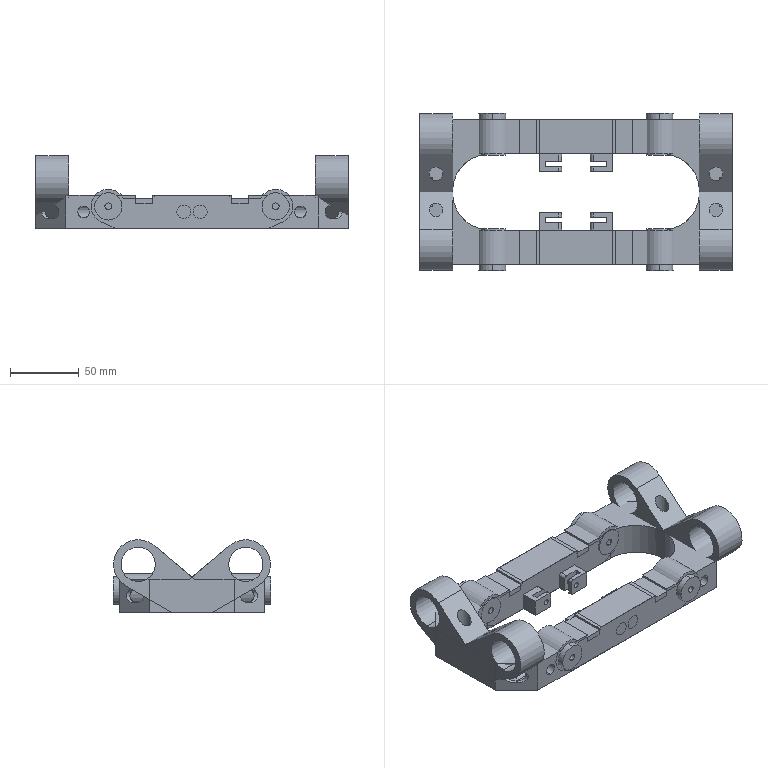NC program | Mastercam | posted with a generic post | part box 228 x 114.503 x 53 mm
Lines 1813 to 2707 of 27132:
(50 FEM |TOOL - 23|DIA. OFF. - 23|LEN. - 23|TOOL DIA. - 50.)
N3680 T23 M6
N3682 G0 G54 G90 X92.548 Y31.5 C0. B0. S5000 M3
N3684 G43 H23 Z50.
N3686 Z5.
N3688 G1 Z-.5 F600.
N3690 X87.548 F4000.
N3692 G3 X82.548 Y26.5 J-5.
N3694 G1 Y2.5
N3696 G2 X57.248 Y-22.8 I-25.3
N3698 G1 X11.069
N3700 X-11.419 Y-41.67
N3702 G2 X-39.252 Y-51.8 I-27.833 J33.17
N3704 X-82.552 Y-8.5 J43.3
N3706 X-60.902 Y28.999 I43.3
N3708 G1 X-21.409 Y51.8
N3710 X57.248
N3712 G2 X82.548 Y26.5 J-25.3
N3714 G1 Y21.5
N3716 G3 X87.548 Y16.5 I5.
N3718 G1 X92.548
N3720 Y31.5
N3722 Z-1. F600.
N3724 X87.548 F4000.
N3726 G3 X82.548 Y26.5 J-5.
N3728 G1 Y2.5
N3730 G2 X57.248 Y-22.8 I-25.3
N3732 G1 X11.069
N3734 X-11.419 Y-41.67
N3736 G2 X-39.252 Y-51.8 I-27.833 J33.17
N3738 X-82.552 Y-8.5 J43.3
N3740 X-60.902 Y28.999 I43.3
N3742 G1 X-21.409 Y51.8
N3744 X57.248
N3746 G2 X82.548 Y26.5 J-25.3
N3748 G1 Y21.5
N3750 G3 X87.548 Y16.5 I5.
N3752 G1 X92.548
N3754 Y31.5
N3756 Z-1.5 F600.
N3758 X87.548 F4000.
N3760 G3 X82.548 Y26.5 J-5.
N3762 G1 Y2.5
N3764 G2 X57.248 Y-22.8 I-25.3
N3766 G1 X11.069
N3768 X-11.419 Y-41.67
N3770 G2 X-39.252 Y-51.8 I-27.833 J33.17
N3772 X-82.552 Y-8.5 J43.3
N3774 X-60.902 Y28.999 I43.3
N3776 G1 X-21.409 Y51.8
N3778 X57.248
N3780 G2 X82.548 Y26.5 J-25.3
N3782 G1 Y21.5
N3784 G3 X87.548 Y16.5 I5.
N3786 G1 X92.548
N3788 Y31.5
N3790 Z-2. F600.
N3792 X87.548 F4000.
N3794 G3 X82.548 Y26.5 J-5.
N3796 G1 Y2.5
N3798 G2 X57.248 Y-22.8 I-25.3
N3800 G1 X11.069
N3802 X-11.419 Y-41.67
N3804 G2 X-39.252 Y-51.8 I-27.833 J33.17
N3806 X-82.552 Y-8.5 J43.3
N3808 X-60.902 Y28.999 I43.3
N3810 G1 X-21.409 Y51.8
N3812 X57.248
N3814 G2 X82.548 Y26.5 J-25.3
N3816 G1 Y21.5
N3818 G3 X87.548 Y16.5 I5.
N3820 G1 X92.548
N3822 Y31.5
N3824 Z-2.5 F600.
N3826 X87.548 F4000.
N3828 G3 X82.548 Y26.5 J-5.
N3830 G1 Y2.5
N3832 G2 X57.248 Y-22.8 I-25.3
N3834 G1 X11.069
N3836 X-11.419 Y-41.67
N3838 G2 X-39.252 Y-51.8 I-27.833 J33.17
N3840 X-82.552 Y-8.5 J43.3
N3842 X-60.902 Y28.999 I43.3
N3844 G1 X-21.409 Y51.8
N3846 X57.248
N3848 G2 X82.548 Y26.5 J-25.3
N3850 G1 Y21.5
N3852 G3 X87.548 Y16.5 I5.
N3854 G1 X92.548
N3856 Y31.5
N3858 Z-3. F600.
N3860 X87.548 F4000.
N3862 G3 X82.548 Y26.5 J-5.
N3864 G1 Y2.5
N3866 G2 X57.248 Y-22.8 I-25.3
N3868 G1 X11.069
N3870 X-11.419 Y-41.67
N3872 G2 X-39.252 Y-51.8 I-27.833 J33.17
N3874 X-82.552 Y-8.5 J43.3
N3876 X-60.902 Y28.999 I43.3
N3878 G1 X-21.409 Y51.8
N3880 X57.248
N3882 G2 X82.548 Y26.5 J-25.3
N3884 G1 Y21.5
N3886 G3 X87.548 Y16.5 I5.
N3888 G1 X92.548
N3890 Y31.5
N3892 Z-3.5 F600.
N3894 X87.548 F4000.
N3896 G3 X82.548 Y26.5 J-5.
N3898 G1 Y2.5
N3900 G2 X57.248 Y-22.8 I-25.3
N3902 G1 X11.069
N3904 X-11.419 Y-41.67
N3906 G2 X-39.252 Y-51.8 I-27.833 J33.17
N3908 X-82.552 Y-8.5 J43.3
N3910 X-60.902 Y28.999 I43.3
N3912 G1 X-21.409 Y51.8
N3914 X57.248
N3916 G2 X82.548 Y26.5 J-25.3
N3918 G1 Y21.5
N3920 G3 X87.548 Y16.5 I5.
N3922 G1 X92.548
N3924 Y31.5
N3926 Z-4. F600.
N3928 X87.548 F4000.
N3930 G3 X82.548 Y26.5 J-5.
N3932 G1 Y2.5
N3934 G2 X57.248 Y-22.8 I-25.3
N3936 G1 X11.069
N3938 X-11.419 Y-41.67
N3940 G2 X-39.252 Y-51.8 I-27.833 J33.17
N3942 X-82.552 Y-8.5 J43.3
N3944 X-60.902 Y28.999 I43.3
N3946 G1 X-21.409 Y51.8
N3948 X57.248
N3950 G2 X82.548 Y26.5 J-25.3
N3952 G1 Y21.5
N3954 G3 X87.548 Y16.5 I5.
N3956 G1 X92.548
N3958 Y31.5
N3960 Z-4.5 F600.
N3962 X87.548 F4000.
N3964 G3 X82.548 Y26.5 J-5.
N3966 G1 Y2.5
N3968 G2 X57.248 Y-22.8 I-25.3
N3970 G1 X11.069
N3972 X-11.419 Y-41.67
N3974 G2 X-39.252 Y-51.8 I-27.833 J33.17
N3976 X-82.552 Y-8.5 J43.3
N3978 X-60.902 Y28.999 I43.3
N3980 G1 X-21.409 Y51.8
N3982 X57.248
N3984 G2 X82.548 Y26.5 J-25.3
N3986 G1 Y21.5
N3988 G3 X87.548 Y16.5 I5.
N3990 G1 X92.548
N3992 Y31.5
N3994 Z-5. F600.
N3996 X87.548 F4000.
N3998 G3 X82.548 Y26.5 J-5.
N4000 G1 Y2.5
N4002 G2 X57.248 Y-22.8 I-25.3
N4004 G1 X11.069
N4006 X-11.419 Y-41.67
N4008 G2 X-39.252 Y-51.8 I-27.833 J33.17
N4010 X-82.552 Y-8.5 J43.3
N4012 X-60.902 Y28.999 I43.3
N4014 G1 X-21.409 Y51.8
N4016 X57.248
N4018 G2 X82.548 Y26.5 J-25.3
N4020 G1 Y21.5
N4022 G3 X87.548 Y16.5 I5.
N4024 G1 X92.548
N4026 Y31.5
N4028 Z-5.5 F600.
N4030 X87.548 F4000.
N4032 G3 X82.548 Y26.5 J-5.
N4034 G1 Y2.5
N4036 G2 X57.248 Y-22.8 I-25.3
N4038 G1 X11.069
N4040 X-11.419 Y-41.67
N4042 G2 X-39.252 Y-51.8 I-27.833 J33.17
N4044 X-82.552 Y-8.5 J43.3
N4046 X-60.902 Y28.999 I43.3
N4048 G1 X-21.409 Y51.8
N4050 X57.248
N4052 G2 X82.548 Y26.5 J-25.3
N4054 G1 Y21.5
N4056 G3 X87.548 Y16.5 I5.
N4058 G1 X92.548
N4060 Y31.5
N4062 Z-6. F600.
N4064 X87.548 F4000.
N4066 G3 X82.548 Y26.5 J-5.
N4068 G1 Y2.5
N4070 G2 X57.248 Y-22.8 I-25.3
N4072 G1 X11.069
N4074 X-11.419 Y-41.67
N4076 G2 X-39.252 Y-51.8 I-27.833 J33.17
N4078 X-82.552 Y-8.5 J43.3
N4080 X-60.902 Y28.999 I43.3
N4082 G1 X-21.409 Y51.8
N4084 X57.248
N4086 G2 X82.548 Y26.5 J-25.3
N4088 G1 Y21.5
N4090 G3 X87.548 Y16.5 I5.
N4092 G1 X92.548
N4094 Y31.5
N4096 Z-6.5 F600.
N4098 X87.548 F4000.
N4100 G3 X82.548 Y26.5 J-5.
N4102 G1 Y2.5
N4104 G2 X57.248 Y-22.8 I-25.3
N4106 G1 X11.069
N4108 X-11.419 Y-41.67
N4110 G2 X-39.252 Y-51.8 I-27.833 J33.17
N4112 X-82.552 Y-8.5 J43.3
N4114 X-60.902 Y28.999 I43.3
N4116 G1 X-21.409 Y51.8
N4118 X57.248
N4120 G2 X82.548 Y26.5 J-25.3
N4122 G1 Y21.5
N4124 G3 X87.548 Y16.5 I5.
N4126 G1 X92.548
N4128 Y31.5
N4130 Z-7. F600.
N4132 X87.548 F4000.
N4134 G3 X82.548 Y26.5 J-5.
N4136 G1 Y2.5
N4138 G2 X57.248 Y-22.8 I-25.3
N4140 G1 X11.069
N4142 X-11.419 Y-41.67
N4144 G2 X-39.252 Y-51.8 I-27.833 J33.17
N4146 X-82.552 Y-8.5 J43.3
N4148 X-60.902 Y28.999 I43.3
N4150 G1 X-21.409 Y51.8
N4152 X57.248
N4154 G2 X82.548 Y26.5 J-25.3
N4156 G1 Y21.5
N4158 G3 X87.548 Y16.5 I5.
N4160 G1 X92.548
N4162 Y31.5
N4164 Z-7.5 F600.
N4166 X87.548 F4000.
N4168 G3 X82.548 Y26.5 J-5.
N4170 G1 Y2.5
N4172 G2 X57.248 Y-22.8 I-25.3
N4174 G1 X11.069
N4176 X-11.419 Y-41.67
N4178 G2 X-39.252 Y-51.8 I-27.833 J33.17
N4180 X-82.552 Y-8.5 J43.3
N4182 X-60.902 Y28.999 I43.3
N4184 G1 X-21.409 Y51.8
N4186 X57.248
N4188 G2 X82.548 Y26.5 J-25.3
N4190 G1 Y21.5
N4192 G3 X87.548 Y16.5 I5.
N4194 G1 X92.548
N4196 Y31.5
N4198 Z-8. F600.
N4200 X87.548 F4000.
N4202 G3 X82.548 Y26.5 J-5.
N4204 G1 Y2.5
N4206 G2 X57.248 Y-22.8 I-25.3
N4208 G1 X11.069
N4210 X-11.419 Y-41.67
N4212 G2 X-39.252 Y-51.8 I-27.833 J33.17
N4214 X-82.552 Y-8.5 J43.3
N4216 X-60.902 Y28.999 I43.3
N4218 G1 X-21.409 Y51.8
N4220 X57.248
N4222 G2 X82.548 Y26.5 J-25.3
N4224 G1 Y21.5
N4226 G3 X87.548 Y16.5 I5.
N4228 G1 X92.548
N4230 Y31.5
N4232 Z-8.5 F600.
N4234 X87.548 F4000.
N4236 G3 X82.548 Y26.5 J-5.
N4238 G1 Y2.5
N4240 G2 X57.248 Y-22.8 I-25.3
N4242 G1 X11.069
N4244 X-11.419 Y-41.67
N4246 G2 X-39.252 Y-51.8 I-27.833 J33.17
N4248 X-82.552 Y-8.5 J43.3
N4250 X-60.902 Y28.999 I43.3
N4252 G1 X-21.409 Y51.8
N4254 X57.248
N4256 G2 X82.548 Y26.5 J-25.3
N4258 G1 Y21.5
N4260 G3 X87.548 Y16.5 I5.
N4262 G1 X92.548
N4264 Y31.5
N4266 Z-9. F600.
N4268 X87.548 F4000.
N4270 G3 X82.548 Y26.5 J-5.
N4272 G1 Y2.5
N4274 G2 X57.248 Y-22.8 I-25.3
N4276 G1 X11.069
N4278 X-11.419 Y-41.67
N4280 G2 X-39.252 Y-51.8 I-27.833 J33.17
N4282 X-82.552 Y-8.5 J43.3
N4284 X-60.902 Y28.999 I43.3
N4286 G1 X-21.409 Y51.8
N4288 X57.248
N4290 G2 X82.548 Y26.5 J-25.3
N4292 G1 Y21.5
N4294 G3 X87.548 Y16.5 I5.
N4296 G1 X92.548
N4298 Y31.5
N4300 Z-9.5 F600.
N4302 X87.548 F4000.
N4304 G3 X82.548 Y26.5 J-5.
N4306 G1 Y2.5
N4308 G2 X57.248 Y-22.8 I-25.3
N4310 G1 X11.069
N4312 X-11.419 Y-41.67
N4314 G2 X-39.252 Y-51.8 I-27.833 J33.17
N4316 X-82.552 Y-8.5 J43.3
N4318 X-60.902 Y28.999 I43.3
N4320 G1 X-21.409 Y51.8
N4322 X57.248
N4324 G2 X82.548 Y26.5 J-25.3
N4326 G1 Y21.5
N4328 G3 X87.548 Y16.5 I5.
N4330 G1 X92.548
N4332 Y31.5
N4334 Z-10. F600.
N4336 X87.548 F4000.
N4338 G3 X82.548 Y26.5 J-5.
N4340 G1 Y2.5
N4342 G2 X57.248 Y-22.8 I-25.3
N4344 G1 X11.069
N4346 X-11.419 Y-41.67
N4348 G2 X-39.252 Y-51.8 I-27.833 J33.17
N4350 X-82.552 Y-8.5 J43.3
N4352 X-60.902 Y28.999 I43.3
N4354 G1 X-21.409 Y51.8
N4356 X57.248
N4358 G2 X82.548 Y26.5 J-25.3
N4360 G1 Y21.5
N4362 G3 X87.548 Y16.5 I5.
N4364 G1 X92.548
N4366 Y31.5
N4368 Z-10.5 F600.
N4370 X87.548 F4000.
N4372 G3 X82.548 Y26.5 J-5.
N4374 G1 Y2.5
N4376 G2 X57.248 Y-22.8 I-25.3
N4378 G1 X11.069
N4380 X-11.419 Y-41.67
N4382 G2 X-39.252 Y-51.8 I-27.833 J33.17
N4384 X-82.552 Y-8.5 J43.3
N4386 X-60.902 Y28.999 I43.3
N4388 G1 X-21.409 Y51.8
N4390 X57.248
N4392 G2 X82.548 Y26.5 J-25.3
N4394 G1 Y21.5
N4396 G3 X87.548 Y16.5 I5.
N4398 G1 X92.548
N4400 Y31.5
N4402 Z-11. F600.
N4404 X87.548 F4000.
N4406 G3 X82.548 Y26.5 J-5.
N4408 G1 Y2.5
N4410 G2 X57.248 Y-22.8 I-25.3
N4412 G1 X11.069
N4414 X-11.419 Y-41.67
N4416 G2 X-39.252 Y-51.8 I-27.833 J33.17
N4418 X-82.552 Y-8.5 J43.3
N4420 X-60.902 Y28.999 I43.3
N4422 G1 X-21.409 Y51.8
N4424 X57.248
N4426 G2 X82.548 Y26.5 J-25.3
N4428 G1 Y21.5
N4430 G3 X87.548 Y16.5 I5.
N4432 G1 X92.548
N4434 Y31.5
N4436 Z-11.5 F600.
N4438 X87.548 F4000.
N4440 G3 X82.548 Y26.5 J-5.
N4442 G1 Y2.5
N4444 G2 X57.248 Y-22.8 I-25.3
N4446 G1 X11.069
N4448 X-11.419 Y-41.67
N4450 G2 X-39.252 Y-51.8 I-27.833 J33.17
N4452 X-82.552 Y-8.5 J43.3
N4454 X-60.902 Y28.999 I43.3
N4456 G1 X-21.409 Y51.8
N4458 X57.248
N4460 G2 X82.548 Y26.5 J-25.3
N4462 G1 Y21.5
N4464 G3 X87.548 Y16.5 I5.
N4466 G1 X92.548
N4468 Y31.5
N4470 Z-12. F600.
N4472 X87.548 F4000.
N4474 G3 X82.548 Y26.5 J-5.
N4476 G1 Y2.5
N4478 G2 X57.248 Y-22.8 I-25.3
N4480 G1 X11.069
N4482 X-11.419 Y-41.67
N4484 G2 X-39.252 Y-51.8 I-27.833 J33.17
N4486 X-82.552 Y-8.5 J43.3
N4488 X-60.902 Y28.999 I43.3
N4490 G1 X-21.409 Y51.8
N4492 X57.248
N4494 G2 X82.548 Y26.5 J-25.3
N4496 G1 Y21.5
N4498 G3 X87.548 Y16.5 I5.
N4500 G1 X92.548
N4502 Y31.5
N4504 Z-12.5 F600.
N4506 X87.548 F4000.
N4508 G3 X82.548 Y26.5 J-5.
N4510 G1 Y2.5
N4512 G2 X57.248 Y-22.8 I-25.3
N4514 G1 X11.069
N4516 X-11.419 Y-41.67
N4518 G2 X-39.252 Y-51.8 I-27.833 J33.17
N4520 X-82.552 Y-8.5 J43.3
N4522 X-60.902 Y28.999 I43.3
N4524 G1 X-21.409 Y51.8
N4526 X57.248
N4528 G2 X82.548 Y26.5 J-25.3
N4530 G1 Y21.5
N4532 G3 X87.548 Y16.5 I5.
N4534 G1 X92.548
N4536 Y31.5
N4538 Z-13. F600.
N4540 X87.548 F4000.
N4542 G3 X82.548 Y26.5 J-5.
N4544 G1 Y2.5
N4546 G2 X57.248 Y-22.8 I-25.3
N4548 G1 X11.069
N4550 X-11.419 Y-41.67
N4552 G2 X-39.252 Y-51.8 I-27.833 J33.17
N4554 X-82.552 Y-8.5 J43.3
N4556 X-60.902 Y28.999 I43.3
N4558 G1 X-21.409 Y51.8
N4560 X57.248
N4562 G2 X82.548 Y26.5 J-25.3
N4564 G1 Y21.5
N4566 G3 X87.548 Y16.5 I5.
N4568 G1 X92.548
N4570 Y31.5
N4572 Z-13.5 F600.
N4574 X87.548 F4000.
N4576 G3 X82.548 Y26.5 J-5.
N4578 G1 Y2.5
N4580 G2 X57.248 Y-22.8 I-25.3
N4582 G1 X11.069
N4584 X-11.419 Y-41.67
N4586 G2 X-39.252 Y-51.8 I-27.833 J33.17
N4588 X-82.552 Y-8.5 J43.3
N4590 X-60.902 Y28.999 I43.3
N4592 G1 X-21.409 Y51.8
N4594 X57.248
N4596 G2 X82.548 Y26.5 J-25.3
N4598 G1 Y21.5
N4600 G3 X87.548 Y16.5 I5.
N4602 G1 X92.548
N4604 Y31.5
N4606 Z-14. F600.
N4608 X87.548 F4000.
N4610 G3 X82.548 Y26.5 J-5.
N4612 G1 Y2.5
N4614 G2 X57.248 Y-22.8 I-25.3
N4616 G1 X11.069
N4618 X-11.419 Y-41.67
N4620 G2 X-39.252 Y-51.8 I-27.833 J33.17
N4622 X-82.552 Y-8.5 J43.3
N4624 X-60.902 Y28.999 I43.3
N4626 G1 X-21.409 Y51.8
N4628 X57.248
N4630 G2 X82.548 Y26.5 J-25.3
N4632 G1 Y21.5
N4634 G3 X87.548 Y16.5 I5.
N4636 G1 X92.548
N4638 Y31.5
N4640 Z-14.5 F600.
N4642 X87.548 F4000.
N4644 G3 X82.548 Y26.5 J-5.
N4646 G1 Y2.5
N4648 G2 X57.248 Y-22.8 I-25.3
N4650 G1 X11.069
N4652 X-11.419 Y-41.67
N4654 G2 X-39.252 Y-51.8 I-27.833 J33.17
N4656 X-82.552 Y-8.5 J43.3
N4658 X-60.902 Y28.999 I43.3
N4660 G1 X-21.409 Y51.8
N4662 X57.248
N4664 G2 X82.548 Y26.5 J-25.3
N4666 G1 Y21.5
N4668 G3 X87.548 Y16.5 I5.
N4670 G1 X92.548
N4672 Y31.5
N4674 Z-15. F600.
N4676 X87.548 F4000.
N4678 G3 X82.548 Y26.5 J-5.
N4680 G1 Y2.5
N4682 G2 X57.248 Y-22.8 I-25.3
N4684 G1 X11.069
N4686 X-11.419 Y-41.67
N4688 G2 X-39.252 Y-51.8 I-27.833 J33.17
N4690 X-82.552 Y-8.5 J43.3
N4692 X-60.902 Y28.999 I43.3
N4694 G1 X-21.409 Y51.8
N4696 X57.248
N4698 G2 X82.548 Y26.5 J-25.3
N4700 G1 Y21.5
N4702 G3 X87.548 Y16.5 I5.
N4704 G1 X92.548
N4706 Y31.5
N4708 Z-15.5 F600.
N4710 X87.548 F4000.
N4712 G3 X82.548 Y26.5 J-5.
N4714 G1 Y2.5
N4716 G2 X57.248 Y-22.8 I-25.3
N4718 G1 X11.069
N4720 X-11.419 Y-41.67
N4722 G2 X-39.252 Y-51.8 I-27.833 J33.17
N4724 X-82.552 Y-8.5 J43.3
N4726 X-60.902 Y28.999 I43.3
N4728 G1 X-21.409 Y51.8
N4730 X57.248
N4732 G2 X82.548 Y26.5 J-25.3
N4734 G1 Y21.5
N4736 G3 X87.548 Y16.5 I5.
N4738 G1 X92.548
N4740 Y31.5
N4742 Z-16. F600.
N4744 X87.548 F4000.
N4746 G3 X82.548 Y26.5 J-5.
N4748 G1 Y2.5
N4750 G2 X57.248 Y-22.8 I-25.3
N4752 G1 X11.069
N4754 X-11.419 Y-41.67
N4756 G2 X-39.252 Y-51.8 I-27.833 J33.17
N4758 X-82.552 Y-8.5 J43.3
N4760 X-60.902 Y28.999 I43.3
N4762 G1 X-21.409 Y51.8
N4764 X57.248
N4766 G2 X82.548 Y26.5 J-25.3
N4768 G1 Y21.5
N4770 G3 X87.548 Y16.5 I5.
N4772 G1 X92.548
N4774 Y31.5
N4776 Z-16.5 F600.
N4778 X87.548 F4000.
N4780 G3 X82.548 Y26.5 J-5.
N4782 G1 Y2.5
N4784 G2 X57.248 Y-22.8 I-25.3
N4786 G1 X11.069
N4788 X-11.419 Y-41.67
N4790 G2 X-39.252 Y-51.8 I-27.833 J33.17
N4792 X-82.552 Y-8.5 J43.3
N4794 X-60.902 Y28.999 I43.3
N4796 G1 X-21.409 Y51.8
N4798 X57.248
N4800 G2 X82.548 Y26.5 J-25.3
N4802 G1 Y21.5
N4804 G3 X87.548 Y16.5 I5.
N4806 G1 X92.548
N4808 Y31.5
N4810 Z-17. F600.
N4812 X87.548 F4000.
N4814 G3 X82.548 Y26.5 J-5.
N4816 G1 Y2.5
N4818 G2 X57.248 Y-22.8 I-25.3
N4820 G1 X11.069
N4822 X-11.419 Y-41.67
N4824 G2 X-39.252 Y-51.8 I-27.833 J33.17
N4826 X-82.552 Y-8.5 J43.3
N4828 X-60.902 Y28.999 I43.3
N4830 G1 X-21.409 Y51.8
N4832 X57.248
N4834 G2 X82.548 Y26.5 J-25.3
N4836 G1 Y21.5
N4838 G3 X87.548 Y16.5 I5.
N4840 G1 X92.548
N4842 Y31.5
N4844 Z-17.5 F600.
N4846 X87.548 F4000.
N4848 G3 X82.548 Y26.5 J-5.
N4850 G1 Y2.5
N4852 G2 X57.248 Y-22.8 I-25.3
N4854 G1 X11.069
N4856 X-11.419 Y-41.67
N4858 G2 X-39.252 Y-51.8 I-27.833 J33.17
N4860 X-82.552 Y-8.5 J43.3
N4862 X-60.902 Y28.999 I43.3
N4864 G1 X-21.409 Y51.8
N4866 X57.248
N4868 G2 X82.548 Y26.5 J-25.3
N4870 G1 Y21.5
N4872 G3 X87.548 Y16.5 I5.
N4874 G1 X92.548
N4876 Y31.5
N4878 Z-18. F600.
N4880 X87.548 F4000.
N4882 G3 X82.548 Y26.5 J-5.
N4884 G1 Y2.5
N4886 G2 X57.248 Y-22.8 I-25.3
N4888 G1 X11.069
N4890 X-11.419 Y-41.67
N4892 G2 X-39.252 Y-51.8 I-27.833 J33.17
N4894 X-82.552 Y-8.5 J43.3
N4896 X-60.902 Y28.999 I43.3
N4898 G1 X-21.409 Y51.8
N4900 X57.248
N4902 G2 X82.548 Y26.5 J-25.3
N4904 G1 Y21.5
N4906 G3 X87.548 Y16.5 I5.
N4908 G1 X92.548
N4910 Y31.5
N4912 Z-18.5 F600.
N4914 X87.548 F4000.
N4916 G3 X82.548 Y26.5 J-5.
N4918 G1 Y2.5
N4920 G2 X57.248 Y-22.8 I-25.3
N4922 G1 X11.069
N4924 X-11.419 Y-41.67
N4926 G2 X-39.252 Y-51.8 I-27.833 J33.17
N4928 X-82.552 Y-8.5 J43.3
N4930 X-60.902 Y28.999 I43.3
N4932 G1 X-21.409 Y51.8
N4934 X57.248
N4936 G2 X82.548 Y26.5 J-25.3
N4938 G1 Y21.5
N4940 G3 X87.548 Y16.5 I5.
N4942 G1 X92.548
N4944 Y31.5
N4946 Z-19. F600.
N4948 X87.548 F4000.
N4950 G3 X82.548 Y26.5 J-5.
N4952 G1 Y2.5
N4954 G2 X57.248 Y-22.8 I-25.3
N4956 G1 X11.069
N4958 X-11.419 Y-41.67
N4960 G2 X-39.252 Y-51.8 I-27.833 J33.17
N4962 X-82.552 Y-8.5 J43.3
N4964 X-60.902 Y28.999 I43.3
N4966 G1 X-21.409 Y51.8
N4968 X57.248
N4970 G2 X82.548 Y26.5 J-25.3
N4972 G1 Y21.5
N4974 G3 X87.548 Y16.5 I5.
N4976 G1 X92.548
N4978 Y31.5
N4980 Z-19.5 F600.
N4982 X87.548 F4000.
N4984 G3 X82.548 Y26.5 J-5.
N4986 G1 Y2.5
N4988 G2 X57.248 Y-22.8 I-25.3
N4990 G1 X11.069
N4992 X-11.419 Y-41.67
N4994 G2 X-39.252 Y-51.8 I-27.833 J33.17
N4996 X-82.552 Y-8.5 J43.3
N4998 X-60.902 Y28.999 I43.3
N5000 G1 X-21.409 Y51.8
N5002 X57.248
N5004 G2 X82.548 Y26.5 J-25.3
N5006 G1 Y21.5
N5008 G3 X87.548 Y16.5 I5.
N5010 G1 X92.548
N5012 Y31.5
N5014 Z-20. F600.
N5016 X87.548 F4000.
N5018 G3 X82.548 Y26.5 J-5.
N5020 G1 Y2.5
N5022 G2 X57.248 Y-22.8 I-25.3
N5024 G1 X11.069
N5026 X-11.419 Y-41.67
N5028 G2 X-39.252 Y-51.8 I-27.833 J33.17
N5030 X-82.552 Y-8.5 J43.3
N5032 X-60.902 Y28.999 I43.3
N5034 G1 X-21.409 Y51.8
N5036 X57.248
N5038 G2 X82.548 Y26.5 J-25.3
N5040 G1 Y21.5
N5042 G3 X87.548 Y16.5 I5.
N5044 G1 X92.548
N5046 Y31.5
N5048 Z-20.5 F600.
N5050 X87.548 F4000.
N5052 G3 X82.548 Y26.5 J-5.
N5054 G1 Y2.5
N5056 G2 X57.248 Y-22.8 I-25.3
N5058 G1 X11.069
N5060 X-11.419 Y-41.67
N5062 G2 X-39.252 Y-51.8 I-27.833 J33.17
N5064 X-82.552 Y-8.5 J43.3
N5066 X-60.902 Y28.999 I43.3
N5068 G1 X-21.409 Y51.8
N5070 X57.248
N5072 G2 X82.548 Y26.5 J-25.3
N5074 G1 Y21.5
N5076 G3 X87.548 Y16.5 I5.
N5078 G1 X92.548
N5080 Y31.5
N5082 Z-21. F600.
N5084 X87.548 F4000.
N5086 G3 X82.548 Y26.5 J-5.
N5088 G1 Y2.5
N5090 G2 X57.248 Y-22.8 I-25.3
N5092 G1 X11.069
N5094 X-11.419 Y-41.67
N5096 G2 X-39.252 Y-51.8 I-27.833 J33.17
N5098 X-82.552 Y-8.5 J43.3
N5100 X-60.902 Y28.999 I43.3
N5102 G1 X-21.409 Y51.8
N5104 X57.248
N5106 G2 X82.548 Y26.5 J-25.3
N5108 G1 Y21.5
N5110 G3 X87.548 Y16.5 I5.
N5112 G1 X92.548
N5114 Y31.5
N5116 Z-21.5 F600.
N5118 X87.548 F4000.
N5120 G3 X82.548 Y26.5 J-5.
N5122 G1 Y2.5
N5124 G2 X57.248 Y-22.8 I-25.3
N5126 G1 X11.069
N5128 X-11.419 Y-41.67
N5130 G2 X-39.252 Y-51.8 I-27.833 J33.17
N5132 X-82.552 Y-8.5 J43.3
N5134 X-60.902 Y28.999 I43.3
N5136 G1 X-21.409 Y51.8
N5138 X57.248
N5140 G2 X82.548 Y26.5 J-25.3
N5142 G1 Y21.5
N5144 G3 X87.548 Y16.5 I5.
N5146 G1 X92.548
N5148 Y31.5
N5150 Z-22. F600.
N5152 X87.548 F4000.
N5154 G3 X82.548 Y26.5 J-5.
N5156 G1 Y2.5
N5158 G2 X57.248 Y-22.8 I-25.3
N5160 G1 X11.069
N5162 X-11.419 Y-41.67
N5164 G2 X-39.252 Y-51.8 I-27.833 J33.17
N5166 X-82.552 Y-8.5 J43.3
N5168 X-60.902 Y28.999 I43.3
N5170 G1 X-21.409 Y51.8
N5172 X57.248
N5174 G2 X82.548 Y26.5 J-25.3
N5176 G1 Y21.5
N5178 G3 X87.548 Y16.5 I5.
N5180 G1 X92.548
N5182 Y31.5
N5184 Z-22.5 F600.
N5186 X87.548 F4000.
N5188 G3 X82.548 Y26.5 J-5.
N5190 G1 Y2.5
N5192 G2 X57.248 Y-22.8 I-25.3
N5194 G1 X11.069
N5196 X-11.419 Y-41.67
N5198 G2 X-39.252 Y-51.8 I-27.833 J33.17
N5200 X-82.552 Y-8.5 J43.3
N5202 X-60.902 Y28.999 I43.3
N5204 G1 X-21.409 Y51.8
N5206 X57.248
N5208 G2 X82.548 Y26.5 J-25.3
N5210 G1 Y21.5
N5212 G3 X87.548 Y16.5 I5.
N5214 G1 X92.548
N5216 Y31.5
N5218 Z-23. F600.
N5220 X87.548 F4000.
N5222 G3 X82.548 Y26.5 J-5.
N5224 G1 Y2.5
N5226 G2 X57.248 Y-22.8 I-25.3
N5228 G1 X11.069
N5230 X-11.419 Y-41.67
N5232 G2 X-39.252 Y-51.8 I-27.833 J33.17
N5234 X-82.552 Y-8.5 J43.3
N5236 X-60.902 Y28.999 I43.3
N5238 G1 X-21.409 Y51.8
N5240 X57.248
N5242 G2 X82.548 Y26.5 J-25.3
N5244 G1 Y21.5
N5246 G3 X87.548 Y16.5 I5.
N5248 G1 X92.548
N5250 Y31.5
N5252 Z-23.5 F600.
N5254 X87.548 F4000.
N5256 G3 X82.548 Y26.5 J-5.
N5258 G1 Y2.5
N5260 G2 X57.248 Y-22.8 I-25.3
N5262 G1 X11.069
N5264 X-11.419 Y-41.67
N5266 G2 X-39.252 Y-51.8 I-27.833 J33.17
N5268 X-82.552 Y-8.5 J43.3
N5270 X-60.902 Y28.999 I43.3
N5272 G1 X-21.409 Y51.8
N5274 X57.248
N5276 G2 X82.548 Y26.5 J-25.3
N5278 G1 Y21.5
N5280 G3 X87.548 Y16.5 I5.
N5282 G1 X92.548
N5284 Y31.5
N5286 Z-24. F600.
N5288 X87.548 F4000.
N5290 G3 X82.548 Y26.5 J-5.
N5292 G1 Y2.5
N5294 G2 X57.248 Y-22.8 I-25.3
N5296 G1 X11.069
N5298 X-11.419 Y-41.67
N5300 G2 X-39.252 Y-51.8 I-27.833 J33.17
N5302 X-82.552 Y-8.5 J43.3
N5304 X-60.902 Y28.999 I43.3
N5306 G1 X-21.409 Y51.8
N5308 X57.248
N5310 G2 X82.548 Y26.5 J-25.3
N5312 G1 Y21.5
N5314 G3 X87.548 Y16.5 I5.
N5316 G1 X92.548
N5318 Y31.5
N5320 Z-24.5 F600.
N5322 X87.548 F4000.
N5324 G3 X82.548 Y26.5 J-5.
N5326 G1 Y2.5
N5328 G2 X57.248 Y-22.8 I-25.3
N5330 G1 X11.069
N5332 X-11.419 Y-41.67
N5334 G2 X-39.252 Y-51.8 I-27.833 J33.17
N5336 X-82.552 Y-8.5 J43.3
N5338 X-60.902 Y28.999 I43.3
N5340 G1 X-21.409 Y51.8
N5342 X57.248
N5344 G2 X82.548 Y26.5 J-25.3
N5346 G1 Y21.5
N5348 G3 X87.548 Y16.5 I5.
N5350 G1 X92.548
N5352 Y31.5
N5354 Z-25. F600.
N5356 X87.548 F4000.
N5358 G3 X82.548 Y26.5 J-5.
N5360 G1 Y2.5
N5362 G2 X57.248 Y-22.8 I-25.3
N5364 G1 X11.069
N5366 X-11.419 Y-41.67
N5368 G2 X-39.252 Y-51.8 I-27.833 J33.17
N5370 X-82.552 Y-8.5 J43.3
N5372 X-60.902 Y28.999 I43.3
N5374 G1 X-21.409 Y51.8
N5376 X57.248
N5378 G2 X82.548 Y26.5 J-25.3
N5380 G1 Y21.5
N5382 G3 X87.548 Y16.5 I5.
N5384 G1 X92.548
N5386 Y31.5
N5388 Z-25.5 F600.
N5390 X87.548 F4000.
N5392 G3 X82.548 Y26.5 J-5.
N5394 G1 Y2.5
N5396 G2 X57.248 Y-22.8 I-25.3
N5398 G1 X11.069
N5400 X-11.419 Y-41.67
N5402 G2 X-39.252 Y-51.8 I-27.833 J33.17
N5404 X-82.552 Y-8.5 J43.3
N5406 X-60.902 Y28.999 I43.3
N5408 G1 X-21.409 Y51.8
N5410 X57.248
N5412 G2 X82.548 Y26.5 J-25.3
N5414 G1 Y21.5
N5416 G3 X87.548 Y16.5 I5.
N5418 G1 X92.548
N5420 Y31.5
N5422 Z-26. F600.
N5424 X87.548 F4000.
N5426 G3 X82.548 Y26.5 J-5.
N5428 G1 Y2.5
N5430 G2 X57.248 Y-22.8 I-25.3
N5432 G1 X11.069
N5434 X-11.419 Y-41.67
N5436 G2 X-39.252 Y-51.8 I-27.833 J33.17
N5438 X-82.552 Y-8.5 J43.3
N5440 X-60.902 Y28.999 I43.3
N5442 G1 X-21.409 Y51.8
N5444 X57.248
N5446 G2 X82.548 Y26.5 J-25.3
N5448 G1 Y21.5
N5450 G3 X87.548 Y16.5 I5.
N5452 G1 X92.548
N5454 G0 Z50.
N5456 M5
N5458 G0 G28 G91 Z0.
N5460 G28
N5462 M01
N5464 G0 G17 G40 G80 G90 G94 G98
N5466 G0 G28 G91 Z0.